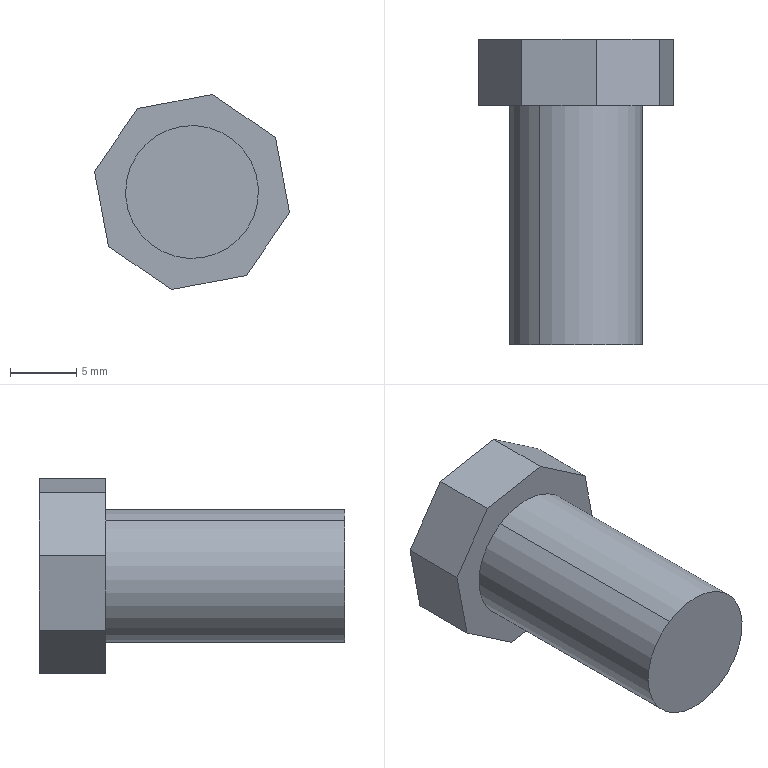Part | SolidWorks | features BaseBody 1 | 1 solid | 13 faces | box 14.681 x 23 x 14.681 mm | volume 2209 mm3 | plane 11 | cylinder 2 | commonest cylinder face diameters 10 x2
STEP:
#1=CARTESIAN_POINT('',(-378.017,-0.8616,-265.814));
#2=VERTEX_POINT('',#1);
#3=CARTESIAN_POINT('',(-372.548,-0.8616,-274.186));
#4=VERTEX_POINT('',#3);
#5=CARTESIAN_POINT('',(-375.282,-0.8616,-270.));
#6=DIRECTION('',(0.,-1.,0.));
#7=DIRECTION('',(-0.5469,0.,0.8372));
#8=AXIS2_PLACEMENT_3D('',#5,#6,#7);
#9=CIRCLE('',#8,5.);
#10=EDGE_CURVE('',#2,#4,#9,.T.);
#11=ORIENTED_EDGE('',*,*,#10,.F.);
#12=CARTESIAN_POINT('',(-378.017,17.138,-265.814));
#13=VERTEX_POINT('',#12);
#14=CARTESIAN_POINT('',(-378.017,-0.8616,-265.814));
#15=DIRECTION('',(0.,1.,0.));
#16=VECTOR('',#15,1000.);
#17=LINE('',#14,#16);
#18=EDGE_CURVE('',#2,#13,#17,.T.);
#19=ORIENTED_EDGE('',*,*,#18,.T.);
#20=CARTESIAN_POINT('',(-372.548,17.138,-274.186));
#21=VERTEX_POINT('',#20);
#22=CARTESIAN_POINT('',(-375.282,17.138,-270.));
#23=DIRECTION('',(0.,-1.,0.));
#24=DIRECTION('',(-0.5469,0.,0.8372));
#25=AXIS2_PLACEMENT_3D('',#22,#23,#24);
#26=CIRCLE('',#25,5.);
#27=EDGE_CURVE('',#13,#21,#26,.T.);
#28=ORIENTED_EDGE('',*,*,#27,.T.);
#29=CARTESIAN_POINT('',(-372.548,-0.8616,-274.186));
#30=DIRECTION('',(0.,1.,0.));
#31=VECTOR('',#30,1000.);
#32=LINE('',#29,#31);
#33=EDGE_CURVE('',#4,#21,#32,.T.);
#34=ORIENTED_EDGE('',*,*,#33,.F.);
#35=EDGE_LOOP('',(#11,#19,#28,#34));
#36=FACE_OUTER_BOUND('',#35,.T.);
#37=CARTESIAN_POINT('',(-375.282,-0.8616,-270.));
#38=DIRECTION('',(0.,1.,0.));
#39=DIRECTION('',(0.5469,0.,-0.8372));
#40=AXIS2_PLACEMENT_3D('',#37,#38,#39);
#41=CYLINDRICAL_SURFACE('',#40,5.);
#42=ADVANCED_FACE('',(#36),#41,.T.);
#43=CARTESIAN_POINT('',(-379.384,17.138,-263.721));
#44=VERTEX_POINT('',#43);
#45=CARTESIAN_POINT('',(-382.623,17.138,-268.461));
#46=VERTEX_POINT('',#45);
#47=CARTESIAN_POINT('',(-379.384,17.138,-263.721));
#48=DIRECTION('',(-0.5641,0.,-0.8257));
#49=VECTOR('',#48,1000.);
#50=LINE('',#47,#49);
#51=EDGE_CURVE('',#44,#46,#50,.T.);
#52=ORIENTED_EDGE('',*,*,#51,.T.);
#53=CARTESIAN_POINT('',(-381.561,17.138,-274.102));
#54=VERTEX_POINT('',#53);
#55=CARTESIAN_POINT('',(-381.561,17.138,-274.102));
#56=DIRECTION('',(0.1849,0.,-0.9827));
#57=VECTOR('',#56,1000.);
#58=LINE('',#55,#57);
#59=EDGE_CURVE('',#46,#54,#58,.T.);
#60=ORIENTED_EDGE('',*,*,#59,.T.);
#61=CARTESIAN_POINT('',(-376.821,17.138,-277.34));
#62=VERTEX_POINT('',#61);
#63=CARTESIAN_POINT('',(-381.561,17.138,-274.102));
#64=DIRECTION('',(0.8257,0.,-0.5641));
#65=VECTOR('',#64,1000.);
#66=LINE('',#63,#65);
#67=EDGE_CURVE('',#54,#62,#66,.T.);
#68=ORIENTED_EDGE('',*,*,#67,.T.);
#69=CARTESIAN_POINT('',(-371.18,17.138,-276.279));
#70=VERTEX_POINT('',#69);
#71=CARTESIAN_POINT('',(-371.18,17.138,-276.279));
#72=DIRECTION('',(0.9827,0.,0.1849));
#73=VECTOR('',#72,1000.);
#74=LINE('',#71,#73);
#75=EDGE_CURVE('',#62,#70,#74,.T.);
#76=ORIENTED_EDGE('',*,*,#75,.T.);
#77=CARTESIAN_POINT('',(-367.942,17.138,-271.539));
#78=VERTEX_POINT('',#77);
#79=CARTESIAN_POINT('',(-371.18,17.138,-276.279));
#80=DIRECTION('',(0.5641,0.,0.8257));
#81=VECTOR('',#80,1000.);
#82=LINE('',#79,#81);
#83=EDGE_CURVE('',#70,#78,#82,.T.);
#84=ORIENTED_EDGE('',*,*,#83,.T.);
#85=CARTESIAN_POINT('',(-369.003,17.138,-265.898));
#86=VERTEX_POINT('',#85);
#87=CARTESIAN_POINT('',(-369.003,17.138,-265.898));
#88=DIRECTION('',(-0.1849,0.,0.9827));
#89=VECTOR('',#88,1000.);
#90=LINE('',#87,#89);
#91=EDGE_CURVE('',#78,#86,#90,.T.);
#92=ORIENTED_EDGE('',*,*,#91,.T.);
#93=CARTESIAN_POINT('',(-373.743,17.138,-262.66));
#94=VERTEX_POINT('',#93);
#95=CARTESIAN_POINT('',(-369.003,17.138,-265.898));
#96=DIRECTION('',(-0.8257,0.,0.5641));
#97=VECTOR('',#96,1000.);
#98=LINE('',#95,#97);
#99=EDGE_CURVE('',#86,#94,#98,.T.);
#100=ORIENTED_EDGE('',*,*,#99,.T.);
#101=CARTESIAN_POINT('',(-379.384,17.138,-263.721));
#102=DIRECTION('',(-0.9827,0.,-0.1849));
#103=VECTOR('',#102,1000.);
#104=LINE('',#101,#103);
#105=EDGE_CURVE('',#94,#44,#104,.T.);
#106=ORIENTED_EDGE('',*,*,#105,.T.);
#107=EDGE_LOOP('',(#52,#60,#68,#76,#84,#92,#100,#106));
#108=FACE_OUTER_BOUND('',#107,.T.);
#109=CARTESIAN_POINT('',(-375.282,17.138,-270.));
#110=DIRECTION('',(0.,-1.,0.));
#111=DIRECTION('',(-0.5469,0.,0.8372));
#112=AXIS2_PLACEMENT_3D('',#109,#110,#111);
#113=CIRCLE('',#112,5.);
#114=EDGE_CURVE('',#21,#13,#113,.T.);
#115=ORIENTED_EDGE('',*,*,#114,.F.);
#116=ORIENTED_EDGE('',*,*,#27,.F.);
#117=EDGE_LOOP('',(#115,#116));
#118=FACE_BOUND('',#117,.T.);
#119=CARTESIAN_POINT('',(-375.282,17.138,-270.));
#120=DIRECTION('',(0.,-1.,0.));
#121=DIRECTION('',(-0.5469,0.,0.8372));
#122=AXIS2_PLACEMENT_3D('',#119,#120,#121);
#123=PLANE('',#122);
#124=ADVANCED_FACE('',(#108,#118),#123,.T.);
#125=CARTESIAN_POINT('',(-379.384,22.138,-263.721));
#126=VERTEX_POINT('',#125);
#127=CARTESIAN_POINT('',(-382.623,22.138,-268.461));
#128=VERTEX_POINT('',#127);
#129=CARTESIAN_POINT('',(-379.384,22.138,-263.721));
#130=DIRECTION('',(-0.5641,0.,-0.8257));
#131=VECTOR('',#130,1000.);
#132=LINE('',#129,#131);
#133=EDGE_CURVE('',#126,#128,#132,.T.);
#134=ORIENTED_EDGE('',*,*,#133,.T.);
#135=CARTESIAN_POINT('',(-382.623,17.138,-268.461));
#136=DIRECTION('',(0.,1.,0.));
#137=VECTOR('',#136,1000.);
#138=LINE('',#135,#137);
#139=EDGE_CURVE('',#46,#128,#138,.T.);
#140=ORIENTED_EDGE('',*,*,#139,.F.);
#141=ORIENTED_EDGE('',*,*,#51,.F.);
#142=CARTESIAN_POINT('',(-379.384,17.138,-263.721));
#143=DIRECTION('',(0.,1.,0.));
#144=VECTOR('',#143,1000.);
#145=LINE('',#142,#144);
#146=EDGE_CURVE('',#44,#126,#145,.T.);
#147=ORIENTED_EDGE('',*,*,#146,.T.);
#148=EDGE_LOOP('',(#134,#140,#141,#147));
#149=FACE_OUTER_BOUND('',#148,.T.);
#150=CARTESIAN_POINT('',(-379.384,17.138,-263.721));
#151=DIRECTION('',(0.8257,0.,-0.5641));
#152=DIRECTION('',(0.5641,0.,0.8257));
#153=AXIS2_PLACEMENT_3D('',#150,#151,#152);
#154=PLANE('',#153);
#155=ADVANCED_FACE('',(#149),#154,.F.);
#156=CARTESIAN_POINT('',(-381.561,22.138,-274.102));
#157=VERTEX_POINT('',#156);
#158=CARTESIAN_POINT('',(-381.561,22.138,-274.102));
#159=DIRECTION('',(0.1849,0.,-0.9827));
#160=VECTOR('',#159,1000.);
#161=LINE('',#158,#160);
#162=EDGE_CURVE('',#128,#157,#161,.T.);
#163=ORIENTED_EDGE('',*,*,#162,.T.);
#164=CARTESIAN_POINT('',(-381.561,17.138,-274.102));
#165=DIRECTION('',(0.,1.,0.));
#166=VECTOR('',#165,1000.);
#167=LINE('',#164,#166);
#168=EDGE_CURVE('',#54,#157,#167,.T.);
#169=ORIENTED_EDGE('',*,*,#168,.F.);
#170=ORIENTED_EDGE('',*,*,#59,.F.);
#171=ORIENTED_EDGE('',*,*,#139,.T.);
#172=EDGE_LOOP('',(#163,#169,#170,#171));
#173=FACE_OUTER_BOUND('',#172,.T.);
#174=CARTESIAN_POINT('',(-381.561,17.138,-274.102));
#175=DIRECTION('',(0.9827,0.,0.1849));
#176=DIRECTION('',(-0.1849,0.,0.9827));
#177=AXIS2_PLACEMENT_3D('',#174,#175,#176);
#178=PLANE('',#177);
#179=ADVANCED_FACE('',(#173),#178,.F.);
#180=CARTESIAN_POINT('',(-376.821,22.138,-277.34));
#181=VERTEX_POINT('',#180);
#182=CARTESIAN_POINT('',(-381.561,22.138,-274.102));
#183=DIRECTION('',(0.8257,0.,-0.5641));
#184=VECTOR('',#183,1000.);
#185=LINE('',#182,#184);
#186=EDGE_CURVE('',#157,#181,#185,.T.);
#187=ORIENTED_EDGE('',*,*,#186,.T.);
#188=CARTESIAN_POINT('',(-376.821,17.138,-277.34));
#189=DIRECTION('',(0.,1.,0.));
#190=VECTOR('',#189,1000.);
#191=LINE('',#188,#190);
#192=EDGE_CURVE('',#62,#181,#191,.T.);
#193=ORIENTED_EDGE('',*,*,#192,.F.);
#194=ORIENTED_EDGE('',*,*,#67,.F.);
#195=ORIENTED_EDGE('',*,*,#168,.T.);
#196=EDGE_LOOP('',(#187,#193,#194,#195));
#197=FACE_OUTER_BOUND('',#196,.T.);
#198=CARTESIAN_POINT('',(-381.561,17.138,-274.102));
#199=DIRECTION('',(0.5641,0.,0.8257));
#200=DIRECTION('',(-0.8257,0.,0.5641));
#201=AXIS2_PLACEMENT_3D('',#198,#199,#200);
#202=PLANE('',#201);
#203=ADVANCED_FACE('',(#197),#202,.F.);
#204=CARTESIAN_POINT('',(-371.18,22.138,-276.279));
#205=VERTEX_POINT('',#204);
#206=CARTESIAN_POINT('',(-371.18,22.138,-276.279));
#207=DIRECTION('',(0.9827,0.,0.1849));
#208=VECTOR('',#207,1000.);
#209=LINE('',#206,#208);
#210=EDGE_CURVE('',#181,#205,#209,.T.);
#211=ORIENTED_EDGE('',*,*,#210,.T.);
#212=CARTESIAN_POINT('',(-371.18,17.138,-276.279));
#213=DIRECTION('',(0.,1.,0.));
#214=VECTOR('',#213,1000.);
#215=LINE('',#212,#214);
#216=EDGE_CURVE('',#70,#205,#215,.T.);
#217=ORIENTED_EDGE('',*,*,#216,.F.);
#218=ORIENTED_EDGE('',*,*,#75,.F.);
#219=ORIENTED_EDGE('',*,*,#192,.T.);
#220=EDGE_LOOP('',(#211,#217,#218,#219));
#221=FACE_OUTER_BOUND('',#220,.T.);
#222=CARTESIAN_POINT('',(-371.18,17.138,-276.279));
#223=DIRECTION('',(-0.1849,0.,0.9827));
#224=DIRECTION('',(-0.9827,0.,-0.1849));
#225=AXIS2_PLACEMENT_3D('',#222,#223,#224);
#226=PLANE('',#225);
#227=ADVANCED_FACE('',(#221),#226,.F.);
#228=CARTESIAN_POINT('',(-367.942,22.138,-271.539));
#229=VERTEX_POINT('',#228);
#230=CARTESIAN_POINT('',(-371.18,22.138,-276.279));
#231=DIRECTION('',(0.5641,0.,0.8257));
#232=VECTOR('',#231,1000.);
#233=LINE('',#230,#232);
#234=EDGE_CURVE('',#205,#229,#233,.T.);
#235=ORIENTED_EDGE('',*,*,#234,.T.);
#236=CARTESIAN_POINT('',(-367.942,17.138,-271.539));
#237=DIRECTION('',(0.,1.,0.));
#238=VECTOR('',#237,1000.);
#239=LINE('',#236,#238);
#240=EDGE_CURVE('',#78,#229,#239,.T.);
#241=ORIENTED_EDGE('',*,*,#240,.F.);
#242=ORIENTED_EDGE('',*,*,#83,.F.);
#243=ORIENTED_EDGE('',*,*,#216,.T.);
#244=EDGE_LOOP('',(#235,#241,#242,#243));
#245=FACE_OUTER_BOUND('',#244,.T.);
#246=CARTESIAN_POINT('',(-371.18,17.138,-276.279));
#247=DIRECTION('',(-0.8257,0.,0.5641));
#248=DIRECTION('',(-0.5641,0.,-0.8257));
#249=AXIS2_PLACEMENT_3D('',#246,#247,#248);
#250=PLANE('',#249);
#251=ADVANCED_FACE('',(#245),#250,.F.);
#252=CARTESIAN_POINT('',(-369.003,22.138,-265.898));
#253=VERTEX_POINT('',#252);
#254=CARTESIAN_POINT('',(-369.003,22.138,-265.898));
#255=DIRECTION('',(-0.1849,0.,0.9827));
#256=VECTOR('',#255,1000.);
#257=LINE('',#254,#256);
#258=EDGE_CURVE('',#229,#253,#257,.T.);
#259=ORIENTED_EDGE('',*,*,#258,.T.);
#260=CARTESIAN_POINT('',(-369.003,17.138,-265.898));
#261=DIRECTION('',(0.,1.,0.));
#262=VECTOR('',#261,1000.);
#263=LINE('',#260,#262);
#264=EDGE_CURVE('',#86,#253,#263,.T.);
#265=ORIENTED_EDGE('',*,*,#264,.F.);
#266=ORIENTED_EDGE('',*,*,#91,.F.);
#267=ORIENTED_EDGE('',*,*,#240,.T.);
#268=EDGE_LOOP('',(#259,#265,#266,#267));
#269=FACE_OUTER_BOUND('',#268,.T.);
#270=CARTESIAN_POINT('',(-369.003,17.138,-265.898));
#271=DIRECTION('',(-0.9827,0.,-0.1849));
#272=DIRECTION('',(0.1849,0.,-0.9827));
#273=AXIS2_PLACEMENT_3D('',#270,#271,#272);
#274=PLANE('',#273);
#275=ADVANCED_FACE('',(#269),#274,.F.);
#276=CARTESIAN_POINT('',(-373.743,22.138,-262.66));
#277=VERTEX_POINT('',#276);
#278=CARTESIAN_POINT('',(-369.003,22.138,-265.898));
#279=DIRECTION('',(-0.8257,0.,0.5641));
#280=VECTOR('',#279,1000.);
#281=LINE('',#278,#280);
#282=EDGE_CURVE('',#253,#277,#281,.T.);
#283=ORIENTED_EDGE('',*,*,#282,.T.);
#284=CARTESIAN_POINT('',(-373.743,17.138,-262.66));
#285=DIRECTION('',(0.,1.,0.));
#286=VECTOR('',#285,1000.);
#287=LINE('',#284,#286);
#288=EDGE_CURVE('',#94,#277,#287,.T.);
#289=ORIENTED_EDGE('',*,*,#288,.F.);
#290=ORIENTED_EDGE('',*,*,#99,.F.);
#291=ORIENTED_EDGE('',*,*,#264,.T.);
#292=EDGE_LOOP('',(#283,#289,#290,#291));
#293=FACE_OUTER_BOUND('',#292,.T.);
#294=CARTESIAN_POINT('',(-369.003,17.138,-265.898));
#295=DIRECTION('',(-0.5641,0.,-0.8257));
#296=DIRECTION('',(0.8257,0.,-0.5641));
#297=AXIS2_PLACEMENT_3D('',#294,#295,#296);
#298=PLANE('',#297);
#299=ADVANCED_FACE('',(#293),#298,.F.);
#300=CARTESIAN_POINT('',(-379.384,22.138,-263.721));
#301=DIRECTION('',(-0.9827,0.,-0.1849));
#302=VECTOR('',#301,1000.);
#303=LINE('',#300,#302);
#304=EDGE_CURVE('',#277,#126,#303,.T.);
#305=ORIENTED_EDGE('',*,*,#304,.T.);
#306=ORIENTED_EDGE('',*,*,#146,.F.);
#307=ORIENTED_EDGE('',*,*,#105,.F.);
#308=ORIENTED_EDGE('',*,*,#288,.T.);
#309=EDGE_LOOP('',(#305,#306,#307,#308));
#310=FACE_OUTER_BOUND('',#309,.T.);
#311=CARTESIAN_POINT('',(-379.384,17.138,-263.721));
#312=DIRECTION('',(0.1849,0.,-0.9827));
#313=DIRECTION('',(0.9827,0.,0.1849));
#314=AXIS2_PLACEMENT_3D('',#311,#312,#313);
#315=PLANE('',#314);
#316=ADVANCED_FACE('',(#310),#315,.F.);
#317=ORIENTED_EDGE('',*,*,#133,.F.);
#318=ORIENTED_EDGE('',*,*,#304,.F.);
#319=ORIENTED_EDGE('',*,*,#282,.F.);
#320=ORIENTED_EDGE('',*,*,#258,.F.);
#321=ORIENTED_EDGE('',*,*,#234,.F.);
#322=ORIENTED_EDGE('',*,*,#210,.F.);
#323=ORIENTED_EDGE('',*,*,#186,.F.);
#324=ORIENTED_EDGE('',*,*,#162,.F.);
#325=EDGE_LOOP('',(#317,#318,#319,#320,#321,#322,#323,#324));
#326=FACE_OUTER_BOUND('',#325,.T.);
#327=CARTESIAN_POINT('',(-375.282,22.138,-270.));
#328=DIRECTION('',(0.,-1.,0.));
#329=DIRECTION('',(-0.5469,0.,0.8372));
#330=AXIS2_PLACEMENT_3D('',#327,#328,#329);
#331=PLANE('',#330);
#332=ADVANCED_FACE('',(#326),#331,.F.);
#333=ORIENTED_EDGE('',*,*,#18,.F.);
#334=CARTESIAN_POINT('',(-375.282,-0.8616,-270.));
#335=DIRECTION('',(0.,-1.,0.));
#336=DIRECTION('',(-0.5469,0.,0.8372));
#337=AXIS2_PLACEMENT_3D('',#334,#335,#336);
#338=CIRCLE('',#337,5.);
#339=EDGE_CURVE('',#4,#2,#338,.T.);
#340=ORIENTED_EDGE('',*,*,#339,.F.);
#341=ORIENTED_EDGE('',*,*,#33,.T.);
#342=ORIENTED_EDGE('',*,*,#114,.T.);
#343=EDGE_LOOP('',(#333,#340,#341,#342));
#344=FACE_OUTER_BOUND('',#343,.T.);
#345=CARTESIAN_POINT('',(-375.282,-0.8616,-270.));
#346=DIRECTION('',(0.,1.,0.));
#347=DIRECTION('',(0.5469,0.,-0.8372));
#348=AXIS2_PLACEMENT_3D('',#345,#346,#347);
#349=CYLINDRICAL_SURFACE('',#348,5.);
#350=ADVANCED_FACE('',(#344),#349,.T.);
#351=ORIENTED_EDGE('',*,*,#339,.T.);
#352=ORIENTED_EDGE('',*,*,#10,.T.);
#353=EDGE_LOOP('',(#351,#352));
#354=FACE_OUTER_BOUND('',#353,.T.);
#355=CARTESIAN_POINT('',(-375.282,-0.8616,-270.));
#356=DIRECTION('',(0.,-1.,0.));
#357=DIRECTION('',(-0.5469,0.,0.8372));
#358=AXIS2_PLACEMENT_3D('',#355,#356,#357);
#359=PLANE('',#358);
#360=ADVANCED_FACE('',(#354),#359,.T.);
#361=CLOSED_SHELL('',(#42,#124,#155,#179,#203,#227,#251,#275,#299,#316,#332,#350,#360));
#362=MANIFOLD_SOLID_BREP('',#361);
#363=CARTESIAN_POINT('',(0.,0.,0.));
#364=DIRECTION('',(0.,0.,1.));
#365=DIRECTION('',(1.,0.,0.));
#366=AXIS2_PLACEMENT_3D('',#363,#364,#365);
#367=(LENGTH_UNIT()NAMED_UNIT(*)SI_UNIT(.MILLI.,.METRE.));
#368=UNCERTAINTY_MEASURE_WITH_UNIT(LENGTH_MEASURE(0.00001),#367,'','');
#369=(NAMED_UNIT(*)PLANE_ANGLE_UNIT()SI_UNIT($,.RADIAN.));
#370=(NAMED_UNIT(*)SI_UNIT($,.STERADIAN.)SOLID_ANGLE_UNIT());
#371=(GEOMETRIC_REPRESENTATION_CONTEXT(3)GLOBAL_UNCERTAINTY_ASSIGNED_CONTEXT((#368))GLOBAL_UNIT_ASSIGNED_CONTEXT((#367,#369,#370))REPRESENTATION_CONTEXT('',''));
#372=ADVANCED_BREP_SHAPE_REPRESENTATION('',(#362,#366),#371);